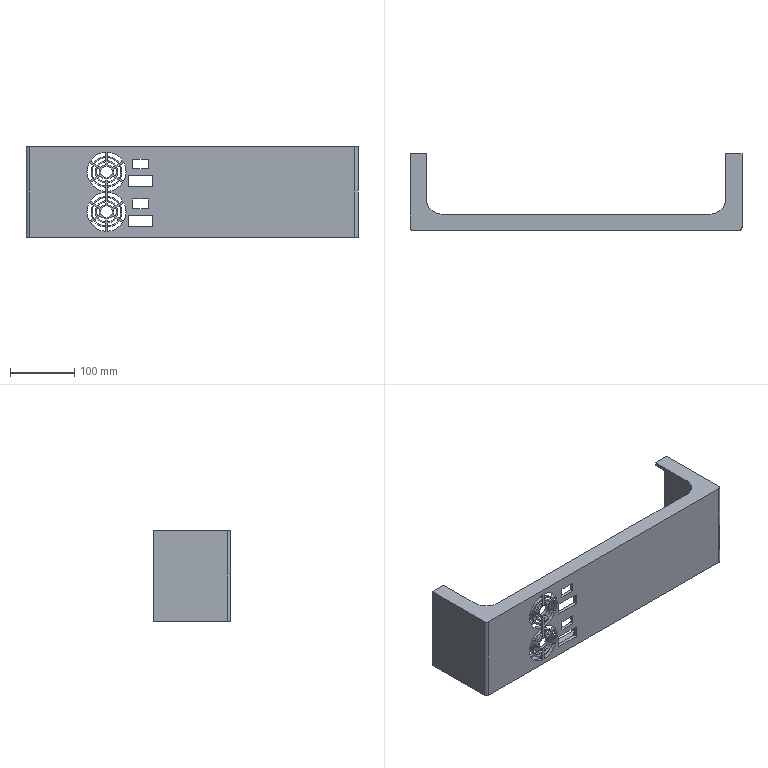Part | NX | features BREP 1 | 1 solid | 188 faces | box 515.254 x 119.165 x 140 mm | volume 630966 mm3 | plane 106 | cylinder 82 | commonest cylinder face diameters 22.181 x12 30.974 x12 34.977 x12 44.307 x12 47.85 x12 60.782 x12